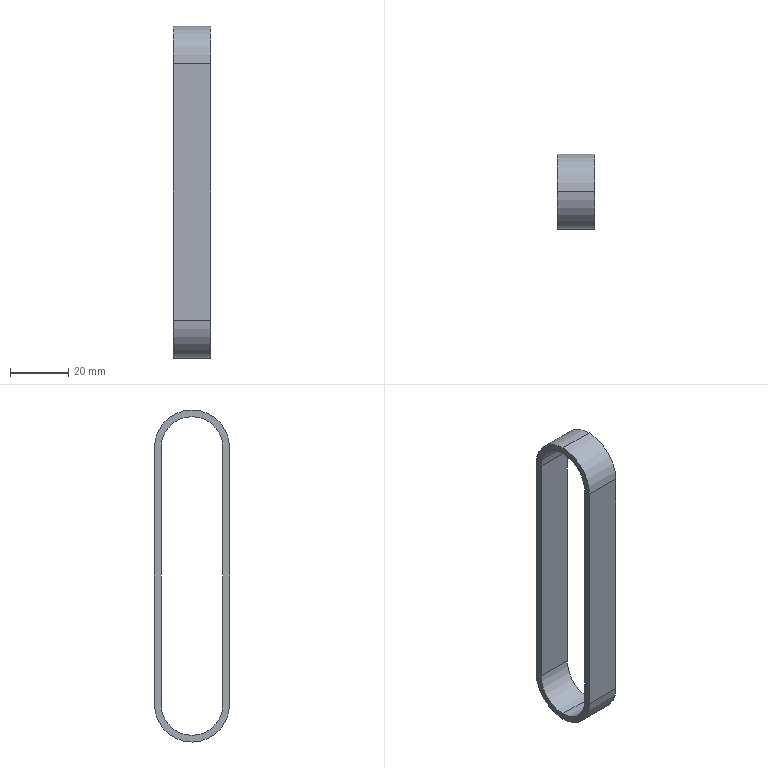Part | NX | features BREP 1 | 1 solid | 14 faces | box 12.7 x 25.75 x 113.73 mm | volume 7199 mm3 | cylinder 8 | plane 6 | commonest cylinder face diameters 21.21 x4 25.75 x4
STEP:
#1=CARTESIAN_POINT('',(6.35,0.,10.605));
#2=VERTEX_POINT('',#1);
#3=CARTESIAN_POINT('',(-6.35,0.,10.605));
#4=VERTEX_POINT('',#3);
#5=CARTESIAN_POINT('',(0.,0.,10.605));
#6=DIRECTION('',(-1.,0.,0.));
#7=VECTOR('',#6,1000.);
#8=LINE('',#5,#7);
#9=EDGE_CURVE('',#2,#4,#8,.T.);
#10=ORIENTED_EDGE('',*,*,#9,.F.);
#11=CARTESIAN_POINT('',(6.35,-10.605,0.));
#12=VERTEX_POINT('',#11);
#13=CARTESIAN_POINT('',(6.35,0.,0.));
#14=DIRECTION('',(-1.,0.,0.));
#15=DIRECTION('',(0.,0.,1.));
#16=AXIS2_PLACEMENT_3D('',#13,#14,#15);
#17=CIRCLE('',#16,10.605);
#18=EDGE_CURVE('',#12,#2,#17,.T.);
#19=ORIENTED_EDGE('',*,*,#18,.F.);
#20=CARTESIAN_POINT('',(-6.35,-10.605,0.));
#21=VERTEX_POINT('',#20);
#22=CARTESIAN_POINT('',(6.35,-10.605,0.));
#23=DIRECTION('',(1.,0.,0.));
#24=VECTOR('',#23,1000.);
#25=LINE('',#22,#24);
#26=EDGE_CURVE('',#21,#12,#25,.T.);
#27=ORIENTED_EDGE('',*,*,#26,.F.);
#28=CARTESIAN_POINT('',(-6.35,0.,0.));
#29=DIRECTION('',(-1.,0.,0.));
#30=DIRECTION('',(0.,0.,1.));
#31=AXIS2_PLACEMENT_3D('',#28,#29,#30);
#32=CIRCLE('',#31,10.605);
#33=EDGE_CURVE('',#21,#4,#32,.T.);
#34=ORIENTED_EDGE('',*,*,#33,.T.);
#35=EDGE_LOOP('',(#10,#19,#27,#34));
#36=FACE_BOUND('',#35,.T.);
#37=CARTESIAN_POINT('',(0.,0.,0.));
#38=DIRECTION('',(-1.,0.,0.));
#39=DIRECTION('',(0.,0.,1.));
#40=AXIS2_PLACEMENT_3D('',#37,#38,#39);
#41=CYLINDRICAL_SURFACE('',#40,10.605);
#42=ADVANCED_FACE('',(#36),#41,.F.);
#43=ORIENTED_EDGE('',*,*,#18,.T.);
#44=CARTESIAN_POINT('',(6.35,10.605,0.));
#45=VERTEX_POINT('',#44);
#46=CARTESIAN_POINT('',(6.35,0.,0.));
#47=DIRECTION('',(-1.,0.,0.));
#48=DIRECTION('',(0.,0.,1.));
#49=AXIS2_PLACEMENT_3D('',#46,#47,#48);
#50=CIRCLE('',#49,10.605);
#51=EDGE_CURVE('',#2,#45,#50,.T.);
#52=ORIENTED_EDGE('',*,*,#51,.T.);
#53=CARTESIAN_POINT('',(6.35,10.605,-87.98));
#54=VERTEX_POINT('',#53);
#55=CARTESIAN_POINT('',(6.35,10.605,-87.98));
#56=DIRECTION('',(0.,0.,1.));
#57=VECTOR('',#56,1000.);
#58=LINE('',#55,#57);
#59=EDGE_CURVE('',#54,#45,#58,.T.);
#60=ORIENTED_EDGE('',*,*,#59,.F.);
#61=CARTESIAN_POINT('',(6.35,0.,-98.585));
#62=VERTEX_POINT('',#61);
#63=CARTESIAN_POINT('',(6.35,0.,-87.98));
#64=DIRECTION('',(1.,0.,0.));
#65=DIRECTION('',(0.,0.,-1.));
#66=AXIS2_PLACEMENT_3D('',#63,#64,#65);
#67=CIRCLE('',#66,10.605);
#68=EDGE_CURVE('',#62,#54,#67,.T.);
#69=ORIENTED_EDGE('',*,*,#68,.F.);
#70=CARTESIAN_POINT('',(6.35,-10.605,-87.98));
#71=VERTEX_POINT('',#70);
#72=CARTESIAN_POINT('',(6.35,0.,-87.98));
#73=DIRECTION('',(1.,0.,0.));
#74=DIRECTION('',(0.,0.,-1.));
#75=AXIS2_PLACEMENT_3D('',#72,#73,#74);
#76=CIRCLE('',#75,10.605);
#77=EDGE_CURVE('',#71,#62,#76,.T.);
#78=ORIENTED_EDGE('',*,*,#77,.F.);
#79=CARTESIAN_POINT('',(6.35,-10.605,0.));
#80=DIRECTION('',(0.,0.,-1.));
#81=VECTOR('',#80,1000.);
#82=LINE('',#79,#81);
#83=EDGE_CURVE('',#12,#71,#82,.T.);
#84=ORIENTED_EDGE('',*,*,#83,.F.);
#85=EDGE_LOOP('',(#43,#52,#60,#69,#78,#84));
#86=FACE_BOUND('',#85,.T.);
#87=CARTESIAN_POINT('',(6.35,-12.875,0.));
#88=VERTEX_POINT('',#87);
#89=CARTESIAN_POINT('',(6.35,0.,12.875));
#90=VERTEX_POINT('',#89);
#91=CARTESIAN_POINT('',(6.35,0.,0.));
#92=DIRECTION('',(-1.,0.,0.));
#93=DIRECTION('',(0.,0.,1.));
#94=AXIS2_PLACEMENT_3D('',#91,#92,#93);
#95=CIRCLE('',#94,12.875);
#96=EDGE_CURVE('',#88,#90,#95,.T.);
#97=ORIENTED_EDGE('',*,*,#96,.F.);
#98=CARTESIAN_POINT('',(6.35,-12.875,-87.98));
#99=VERTEX_POINT('',#98);
#100=CARTESIAN_POINT('',(6.35,-12.875,0.));
#101=DIRECTION('',(0.,0.,-1.));
#102=VECTOR('',#101,1000.);
#103=LINE('',#100,#102);
#104=EDGE_CURVE('',#88,#99,#103,.T.);
#105=ORIENTED_EDGE('',*,*,#104,.T.);
#106=CARTESIAN_POINT('',(6.35,0.,-100.855));
#107=VERTEX_POINT('',#106);
#108=CARTESIAN_POINT('',(6.35,0.,-87.98));
#109=DIRECTION('',(1.,0.,0.));
#110=DIRECTION('',(0.,0.,-1.));
#111=AXIS2_PLACEMENT_3D('',#108,#109,#110);
#112=CIRCLE('',#111,12.875);
#113=EDGE_CURVE('',#99,#107,#112,.T.);
#114=ORIENTED_EDGE('',*,*,#113,.T.);
#115=CARTESIAN_POINT('',(6.35,12.875,-87.98));
#116=VERTEX_POINT('',#115);
#117=CARTESIAN_POINT('',(6.35,0.,-87.98));
#118=DIRECTION('',(1.,0.,0.));
#119=DIRECTION('',(0.,0.,-1.));
#120=AXIS2_PLACEMENT_3D('',#117,#118,#119);
#121=CIRCLE('',#120,12.875);
#122=EDGE_CURVE('',#107,#116,#121,.T.);
#123=ORIENTED_EDGE('',*,*,#122,.T.);
#124=CARTESIAN_POINT('',(6.35,12.875,0.));
#125=VERTEX_POINT('',#124);
#126=CARTESIAN_POINT('',(6.35,12.875,-87.98));
#127=DIRECTION('',(0.,0.,1.));
#128=VECTOR('',#127,1000.);
#129=LINE('',#126,#128);
#130=EDGE_CURVE('',#116,#125,#129,.T.);
#131=ORIENTED_EDGE('',*,*,#130,.T.);
#132=CARTESIAN_POINT('',(6.35,0.,0.));
#133=DIRECTION('',(-1.,0.,0.));
#134=DIRECTION('',(0.,0.,1.));
#135=AXIS2_PLACEMENT_3D('',#132,#133,#134);
#136=CIRCLE('',#135,12.875);
#137=EDGE_CURVE('',#90,#125,#136,.T.);
#138=ORIENTED_EDGE('',*,*,#137,.F.);
#139=EDGE_LOOP('',(#97,#105,#114,#123,#131,#138));
#140=FACE_BOUND('',#139,.T.);
#141=CARTESIAN_POINT('',(6.35,-12.875,0.));
#142=DIRECTION('',(-1.,0.,0.));
#143=DIRECTION('',(0.,0.,1.));
#144=AXIS2_PLACEMENT_3D('',#141,#142,#143);
#145=PLANE('',#144);
#146=ADVANCED_FACE('',(#86,#140),#145,.F.);
#147=CARTESIAN_POINT('',(-6.35,0.,12.875));
#148=VERTEX_POINT('',#147);
#149=CARTESIAN_POINT('',(0.,0.,12.875));
#150=DIRECTION('',(-1.,0.,0.));
#151=VECTOR('',#150,1000.);
#152=LINE('',#149,#151);
#153=EDGE_CURVE('',#90,#148,#152,.T.);
#154=ORIENTED_EDGE('',*,*,#153,.F.);
#155=ORIENTED_EDGE('',*,*,#137,.T.);
#156=CARTESIAN_POINT('',(-6.35,12.875,0.));
#157=VERTEX_POINT('',#156);
#158=CARTESIAN_POINT('',(6.35,12.875,0.));
#159=CARTESIAN_POINT('',(2.117,12.875,0.));
#160=CARTESIAN_POINT('',(-2.117,12.875,0.));
#161=CARTESIAN_POINT('',(-6.35,12.875,0.));
#162=B_SPLINE_CURVE_WITH_KNOTS('',3,(#158,#159,#160,#161),.UNSPECIFIED.,.F.,.F.,(4,4),(0.,1.),.UNSPECIFIED.);
#163=EDGE_CURVE('',#125,#157,#162,.T.);
#164=ORIENTED_EDGE('',*,*,#163,.T.);
#165=CARTESIAN_POINT('',(-6.35,0.,0.));
#166=DIRECTION('',(-1.,0.,0.));
#167=DIRECTION('',(0.,0.,1.));
#168=AXIS2_PLACEMENT_3D('',#165,#166,#167);
#169=CIRCLE('',#168,12.875);
#170=EDGE_CURVE('',#148,#157,#169,.T.);
#171=ORIENTED_EDGE('',*,*,#170,.F.);
#172=EDGE_LOOP('',(#154,#155,#164,#171));
#173=FACE_BOUND('',#172,.T.);
#174=CARTESIAN_POINT('',(0.,0.,0.));
#175=DIRECTION('',(-1.,0.,0.));
#176=DIRECTION('',(0.,0.,1.));
#177=AXIS2_PLACEMENT_3D('',#174,#175,#176);
#178=CYLINDRICAL_SURFACE('',#177,12.875);
#179=ADVANCED_FACE('',(#173),#178,.T.);
#180=CARTESIAN_POINT('',(-6.35,-12.875,0.));
#181=VERTEX_POINT('',#180);
#182=CARTESIAN_POINT('',(-6.35,0.,0.));
#183=DIRECTION('',(-1.,0.,0.));
#184=DIRECTION('',(0.,0.,1.));
#185=AXIS2_PLACEMENT_3D('',#182,#183,#184);
#186=CIRCLE('',#185,12.875);
#187=EDGE_CURVE('',#181,#148,#186,.T.);
#188=ORIENTED_EDGE('',*,*,#187,.T.);
#189=ORIENTED_EDGE('',*,*,#170,.T.);
#190=CARTESIAN_POINT('',(-6.35,12.875,-87.98));
#191=VERTEX_POINT('',#190);
#192=CARTESIAN_POINT('',(-6.35,12.875,-87.98));
#193=DIRECTION('',(0.,0.,1.));
#194=VECTOR('',#193,1000.);
#195=LINE('',#192,#194);
#196=EDGE_CURVE('',#191,#157,#195,.T.);
#197=ORIENTED_EDGE('',*,*,#196,.F.);
#198=CARTESIAN_POINT('',(-6.35,0.,-100.855));
#199=VERTEX_POINT('',#198);
#200=CARTESIAN_POINT('',(-6.35,0.,-87.98));
#201=DIRECTION('',(1.,0.,0.));
#202=DIRECTION('',(0.,0.,-1.));
#203=AXIS2_PLACEMENT_3D('',#200,#201,#202);
#204=CIRCLE('',#203,12.875);
#205=EDGE_CURVE('',#199,#191,#204,.T.);
#206=ORIENTED_EDGE('',*,*,#205,.F.);
#207=CARTESIAN_POINT('',(-6.35,-12.875,-87.98));
#208=VERTEX_POINT('',#207);
#209=CARTESIAN_POINT('',(-6.35,0.,-87.98));
#210=DIRECTION('',(1.,0.,0.));
#211=DIRECTION('',(0.,0.,-1.));
#212=AXIS2_PLACEMENT_3D('',#209,#210,#211);
#213=CIRCLE('',#212,12.875);
#214=EDGE_CURVE('',#208,#199,#213,.T.);
#215=ORIENTED_EDGE('',*,*,#214,.F.);
#216=CARTESIAN_POINT('',(-6.35,-12.875,0.));
#217=DIRECTION('',(0.,0.,-1.));
#218=VECTOR('',#217,1000.);
#219=LINE('',#216,#218);
#220=EDGE_CURVE('',#181,#208,#219,.T.);
#221=ORIENTED_EDGE('',*,*,#220,.F.);
#222=EDGE_LOOP('',(#188,#189,#197,#206,#215,#221));
#223=FACE_BOUND('',#222,.T.);
#224=ORIENTED_EDGE('',*,*,#33,.F.);
#225=CARTESIAN_POINT('',(-6.35,-10.605,-87.98));
#226=VERTEX_POINT('',#225);
#227=CARTESIAN_POINT('',(-6.35,-10.605,0.));
#228=DIRECTION('',(0.,0.,-1.));
#229=VECTOR('',#228,1000.);
#230=LINE('',#227,#229);
#231=EDGE_CURVE('',#21,#226,#230,.T.);
#232=ORIENTED_EDGE('',*,*,#231,.T.);
#233=CARTESIAN_POINT('',(-6.35,0.,-98.585));
#234=VERTEX_POINT('',#233);
#235=CARTESIAN_POINT('',(-6.35,0.,-87.98));
#236=DIRECTION('',(1.,0.,0.));
#237=DIRECTION('',(0.,0.,-1.));
#238=AXIS2_PLACEMENT_3D('',#235,#236,#237);
#239=CIRCLE('',#238,10.605);
#240=EDGE_CURVE('',#226,#234,#239,.T.);
#241=ORIENTED_EDGE('',*,*,#240,.T.);
#242=CARTESIAN_POINT('',(-6.35,10.605,-87.98));
#243=VERTEX_POINT('',#242);
#244=CARTESIAN_POINT('',(-6.35,0.,-87.98));
#245=DIRECTION('',(1.,0.,0.));
#246=DIRECTION('',(0.,0.,-1.));
#247=AXIS2_PLACEMENT_3D('',#244,#245,#246);
#248=CIRCLE('',#247,10.605);
#249=EDGE_CURVE('',#234,#243,#248,.T.);
#250=ORIENTED_EDGE('',*,*,#249,.T.);
#251=CARTESIAN_POINT('',(-6.35,10.605,0.));
#252=VERTEX_POINT('',#251);
#253=CARTESIAN_POINT('',(-6.35,10.605,-87.98));
#254=DIRECTION('',(0.,0.,1.));
#255=VECTOR('',#254,1000.);
#256=LINE('',#253,#255);
#257=EDGE_CURVE('',#243,#252,#256,.T.);
#258=ORIENTED_EDGE('',*,*,#257,.T.);
#259=CARTESIAN_POINT('',(-6.35,0.,0.));
#260=DIRECTION('',(-1.,0.,0.));
#261=DIRECTION('',(0.,0.,1.));
#262=AXIS2_PLACEMENT_3D('',#259,#260,#261);
#263=CIRCLE('',#262,10.605);
#264=EDGE_CURVE('',#4,#252,#263,.T.);
#265=ORIENTED_EDGE('',*,*,#264,.F.);
#266=EDGE_LOOP('',(#224,#232,#241,#250,#258,#265));
#267=FACE_BOUND('',#266,.T.);
#268=CARTESIAN_POINT('',(-6.35,-10.605,0.));
#269=DIRECTION('',(1.,0.,0.));
#270=DIRECTION('',(0.,0.,-1.));
#271=AXIS2_PLACEMENT_3D('',#268,#269,#270);
#272=PLANE('',#271);
#273=ADVANCED_FACE('',(#223,#267),#272,.F.);
#274=CARTESIAN_POINT('',(-6.35,-12.875,0.));
#275=DIRECTION('',(-1.,0.,0.));
#276=VECTOR('',#275,1000.);
#277=LINE('',#274,#276);
#278=EDGE_CURVE('',#88,#181,#277,.T.);
#279=ORIENTED_EDGE('',*,*,#278,.T.);
#280=ORIENTED_EDGE('',*,*,#220,.T.);
#281=CARTESIAN_POINT('',(-6.35,-12.875,-87.98));
#282=DIRECTION('',(-1.,0.,0.));
#283=VECTOR('',#282,1000.);
#284=LINE('',#281,#283);
#285=EDGE_CURVE('',#99,#208,#284,.T.);
#286=ORIENTED_EDGE('',*,*,#285,.F.);
#287=ORIENTED_EDGE('',*,*,#104,.F.);
#288=EDGE_LOOP('',(#279,#280,#286,#287));
#289=FACE_BOUND('',#288,.T.);
#290=CARTESIAN_POINT('',(-6.35,-12.875,0.));
#291=DIRECTION('',(0.,-1.,0.));
#292=DIRECTION('',(0.,0.,-1.));
#293=AXIS2_PLACEMENT_3D('',#290,#291,#292);
#294=PLANE('',#293);
#295=ADVANCED_FACE('',(#289),#294,.T.);
#296=ORIENTED_EDGE('',*,*,#26,.T.);
#297=ORIENTED_EDGE('',*,*,#83,.T.);
#298=CARTESIAN_POINT('',(6.35,-10.605,-87.98));
#299=DIRECTION('',(1.,0.,0.));
#300=VECTOR('',#299,1000.);
#301=LINE('',#298,#300);
#302=EDGE_CURVE('',#226,#71,#301,.T.);
#303=ORIENTED_EDGE('',*,*,#302,.F.);
#304=ORIENTED_EDGE('',*,*,#231,.F.);
#305=EDGE_LOOP('',(#296,#297,#303,#304));
#306=FACE_BOUND('',#305,.T.);
#307=CARTESIAN_POINT('',(6.35,-10.605,0.));
#308=DIRECTION('',(0.,1.,0.));
#309=DIRECTION('',(0.,0.,1.));
#310=AXIS2_PLACEMENT_3D('',#307,#308,#309);
#311=PLANE('',#310);
#312=ADVANCED_FACE('',(#306),#311,.T.);
#313=CARTESIAN_POINT('',(0.,0.,-100.855));
#314=DIRECTION('',(1.,0.,0.));
#315=VECTOR('',#314,1000.);
#316=LINE('',#313,#315);
#317=EDGE_CURVE('',#199,#107,#316,.T.);
#318=ORIENTED_EDGE('',*,*,#317,.F.);
#319=ORIENTED_EDGE('',*,*,#205,.T.);
#320=CARTESIAN_POINT('',(-6.35,12.875,-87.98));
#321=DIRECTION('',(-1.,0.,0.));
#322=VECTOR('',#321,1000.);
#323=LINE('',#320,#322);
#324=EDGE_CURVE('',#116,#191,#323,.T.);
#325=ORIENTED_EDGE('',*,*,#324,.F.);
#326=ORIENTED_EDGE('',*,*,#122,.F.);
#327=EDGE_LOOP('',(#318,#319,#325,#326));
#328=FACE_BOUND('',#327,.T.);
#329=CARTESIAN_POINT('',(0.,0.,-87.98));
#330=DIRECTION('',(1.,0.,0.));
#331=DIRECTION('',(0.,0.,-1.));
#332=AXIS2_PLACEMENT_3D('',#329,#330,#331);
#333=CYLINDRICAL_SURFACE('',#332,12.875);
#334=ADVANCED_FACE('',(#328),#333,.T.);
#335=CARTESIAN_POINT('',(0.,0.,-98.585));
#336=DIRECTION('',(1.,0.,0.));
#337=VECTOR('',#336,1000.);
#338=LINE('',#335,#337);
#339=EDGE_CURVE('',#234,#62,#338,.T.);
#340=ORIENTED_EDGE('',*,*,#339,.F.);
#341=ORIENTED_EDGE('',*,*,#240,.F.);
#342=ORIENTED_EDGE('',*,*,#302,.T.);
#343=ORIENTED_EDGE('',*,*,#77,.T.);
#344=EDGE_LOOP('',(#340,#341,#342,#343));
#345=FACE_BOUND('',#344,.T.);
#346=CARTESIAN_POINT('',(0.,0.,-87.98));
#347=DIRECTION('',(1.,0.,0.));
#348=DIRECTION('',(0.,0.,-1.));
#349=AXIS2_PLACEMENT_3D('',#346,#347,#348);
#350=CYLINDRICAL_SURFACE('',#349,10.605);
#351=ADVANCED_FACE('',(#345),#350,.F.);
#352=ORIENTED_EDGE('',*,*,#324,.T.);
#353=ORIENTED_EDGE('',*,*,#196,.T.);
#354=ORIENTED_EDGE('',*,*,#163,.F.);
#355=ORIENTED_EDGE('',*,*,#130,.F.);
#356=EDGE_LOOP('',(#352,#353,#354,#355));
#357=FACE_BOUND('',#356,.T.);
#358=CARTESIAN_POINT('',(-6.35,12.875,-87.98));
#359=DIRECTION('',(0.,1.,0.));
#360=DIRECTION('',(0.,0.,1.));
#361=AXIS2_PLACEMENT_3D('',#358,#359,#360);
#362=PLANE('',#361);
#363=ADVANCED_FACE('',(#357),#362,.T.);
#364=CARTESIAN_POINT('',(6.35,10.605,-87.98));
#365=DIRECTION('',(1.,0.,0.));
#366=VECTOR('',#365,1000.);
#367=LINE('',#364,#366);
#368=EDGE_CURVE('',#243,#54,#367,.T.);
#369=ORIENTED_EDGE('',*,*,#368,.T.);
#370=ORIENTED_EDGE('',*,*,#59,.T.);
#371=CARTESIAN_POINT('',(-6.35,10.605,0.));
#372=CARTESIAN_POINT('',(-2.117,10.605,0.));
#373=CARTESIAN_POINT('',(2.117,10.605,0.));
#374=CARTESIAN_POINT('',(6.35,10.605,0.));
#375=B_SPLINE_CURVE_WITH_KNOTS('',3,(#371,#372,#373,#374),.UNSPECIFIED.,.F.,.F.,(4,4),(0.,1.),.UNSPECIFIED.);
#376=EDGE_CURVE('',#252,#45,#375,.T.);
#377=ORIENTED_EDGE('',*,*,#376,.F.);
#378=ORIENTED_EDGE('',*,*,#257,.F.);
#379=EDGE_LOOP('',(#369,#370,#377,#378));
#380=FACE_BOUND('',#379,.T.);
#381=CARTESIAN_POINT('',(6.35,10.605,-87.98));
#382=DIRECTION('',(0.,-1.,0.));
#383=DIRECTION('',(0.,0.,-1.));
#384=AXIS2_PLACEMENT_3D('',#381,#382,#383);
#385=PLANE('',#384);
#386=ADVANCED_FACE('',(#380),#385,.T.);
#387=ORIENTED_EDGE('',*,*,#249,.F.);
#388=ORIENTED_EDGE('',*,*,#339,.T.);
#389=ORIENTED_EDGE('',*,*,#68,.T.);
#390=ORIENTED_EDGE('',*,*,#368,.F.);
#391=EDGE_LOOP('',(#387,#388,#389,#390));
#392=FACE_BOUND('',#391,.T.);
#393=CARTESIAN_POINT('',(0.,0.,-87.98));
#394=DIRECTION('',(1.,0.,0.));
#395=DIRECTION('',(0.,0.,-1.));
#396=AXIS2_PLACEMENT_3D('',#393,#394,#395);
#397=CYLINDRICAL_SURFACE('',#396,10.605);
#398=ADVANCED_FACE('',(#392),#397,.F.);
#399=ORIENTED_EDGE('',*,*,#214,.T.);
#400=ORIENTED_EDGE('',*,*,#317,.T.);
#401=ORIENTED_EDGE('',*,*,#113,.F.);
#402=ORIENTED_EDGE('',*,*,#285,.T.);
#403=EDGE_LOOP('',(#399,#400,#401,#402));
#404=FACE_BOUND('',#403,.T.);
#405=CARTESIAN_POINT('',(0.,0.,-87.98));
#406=DIRECTION('',(1.,0.,0.));
#407=DIRECTION('',(0.,0.,-1.));
#408=AXIS2_PLACEMENT_3D('',#405,#406,#407);
#409=CYLINDRICAL_SURFACE('',#408,12.875);
#410=ADVANCED_FACE('',(#404),#409,.T.);
#411=ORIENTED_EDGE('',*,*,#96,.T.);
#412=ORIENTED_EDGE('',*,*,#153,.T.);
#413=ORIENTED_EDGE('',*,*,#187,.F.);
#414=ORIENTED_EDGE('',*,*,#278,.F.);
#415=EDGE_LOOP('',(#411,#412,#413,#414));
#416=FACE_BOUND('',#415,.T.);
#417=CARTESIAN_POINT('',(0.,0.,0.));
#418=DIRECTION('',(-1.,0.,0.));
#419=DIRECTION('',(0.,0.,1.));
#420=AXIS2_PLACEMENT_3D('',#417,#418,#419);
#421=CYLINDRICAL_SURFACE('',#420,12.875);
#422=ADVANCED_FACE('',(#416),#421,.T.);
#423=ORIENTED_EDGE('',*,*,#51,.F.);
#424=ORIENTED_EDGE('',*,*,#9,.T.);
#425=ORIENTED_EDGE('',*,*,#264,.T.);
#426=ORIENTED_EDGE('',*,*,#376,.T.);
#427=EDGE_LOOP('',(#423,#424,#425,#426));
#428=FACE_BOUND('',#427,.T.);
#429=CARTESIAN_POINT('',(0.,0.,0.));
#430=DIRECTION('',(-1.,0.,0.));
#431=DIRECTION('',(0.,0.,1.));
#432=AXIS2_PLACEMENT_3D('',#429,#430,#431);
#433=CYLINDRICAL_SURFACE('',#432,10.605);
#434=ADVANCED_FACE('',(#428),#433,.F.);
#435=CLOSED_SHELL('',(#42,#146,#179,#273,#295,#312,#334,#351,#363,#386,#398,#410,#422,#434));
#436=MANIFOLD_SOLID_BREP('',#435);
#437=(LENGTH_UNIT()NAMED_UNIT(*)SI_UNIT(.MILLI.,.METRE.));
#438=UNCERTAINTY_MEASURE_WITH_UNIT(LENGTH_MEASURE(0.00001),#437,'','');
#439=(NAMED_UNIT(*)PLANE_ANGLE_UNIT()SI_UNIT($,.RADIAN.));
#440=(NAMED_UNIT(*)SI_UNIT($,.STERADIAN.)SOLID_ANGLE_UNIT());
#441=(GEOMETRIC_REPRESENTATION_CONTEXT(3)GLOBAL_UNCERTAINTY_ASSIGNED_CONTEXT((#438))GLOBAL_UNIT_ASSIGNED_CONTEXT((#437,#439,#440))REPRESENTATION_CONTEXT('',''));
#442=ADVANCED_BREP_SHAPE_REPRESENTATION('',(#436),#441);